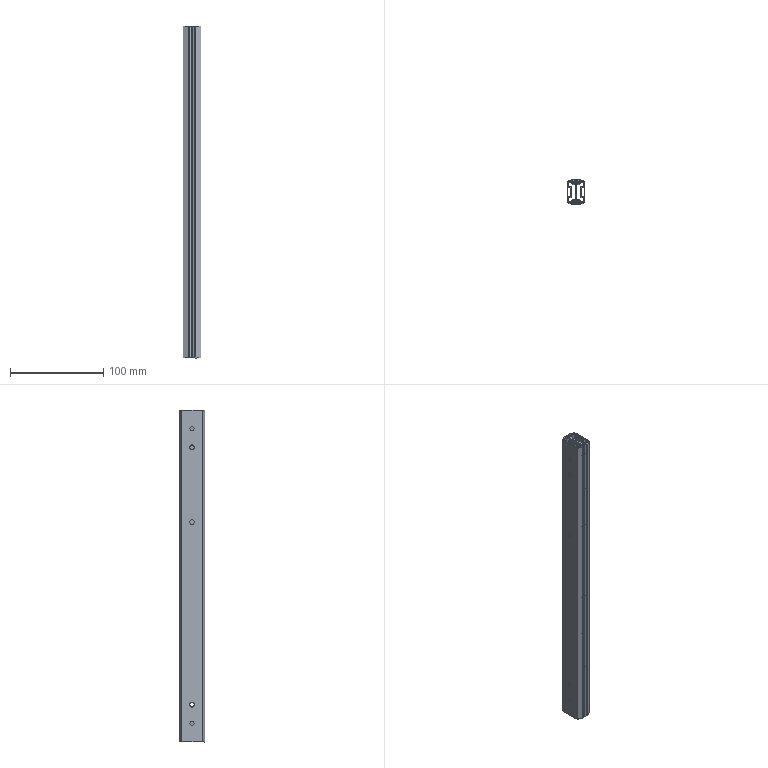Part | SolidWorks | features AEMSimFeature 1 | 5 solids | 275 faces | box 19.1 x 27 x 355.6 mm | volume 53806 mm3 | plane 102 | spline 98 | cylinder 75 | commonest cylinder face diameters 4.5 x36 3.7 x12 9 x12 1 x4 2 x4 3.8 x4